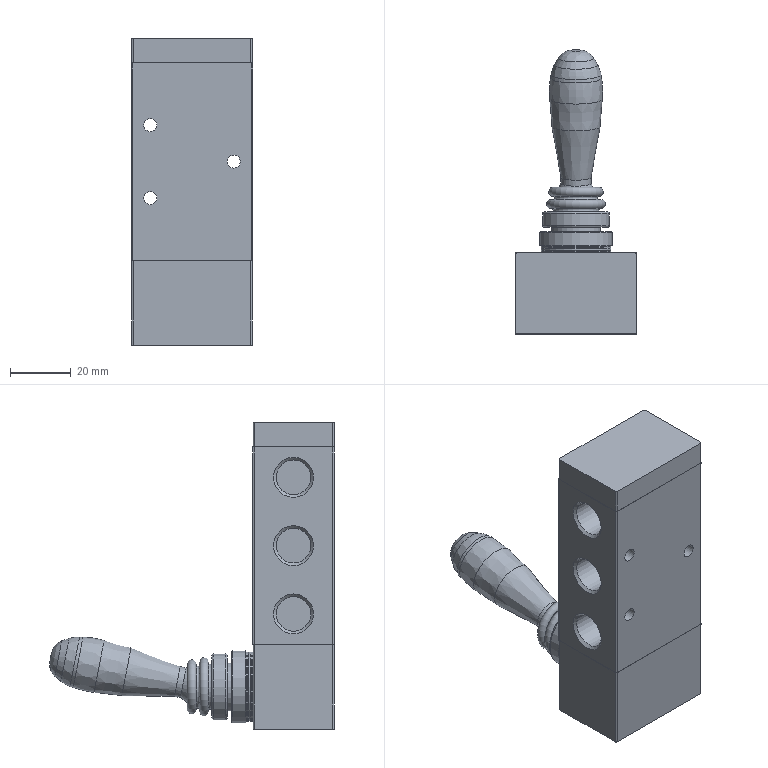Part | STEP file | _4H310PA-08_BODY_id414_x_t | 1 solid | 83 faces | box 40 x 93.887 x 101 mm | volume 115907 mm3 | plane 29 | cylinder 28 | cone 17 | torus 6 | spline 3 | commonest cylinder face diameters 1 x12 11.445 x5 4.3 x3 23 x3 10 x1 12 x1